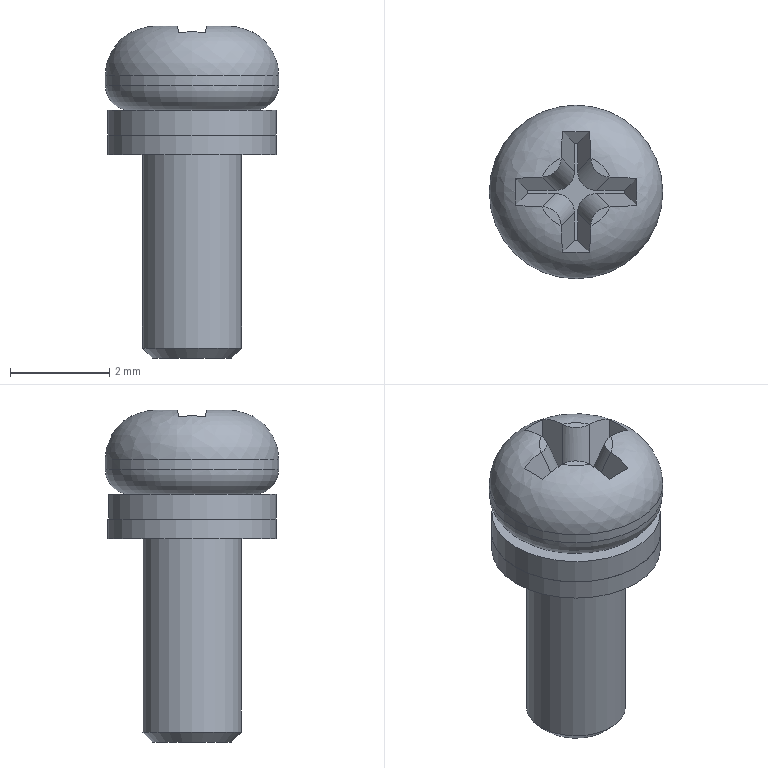Part | STEP file | Pan head combination screw M2X5 | 3 solids | 39 faces | box 3.5 x 3.5 x 6.7 mm | volume 32.079 mm3 | plane 25 | cylinder 10 | torus 2 | spline 1 | cone 1 | commonest cylinder face diameters 0.8 x4 2 x2 3.4 x2 2.6 x1 3.5 x1